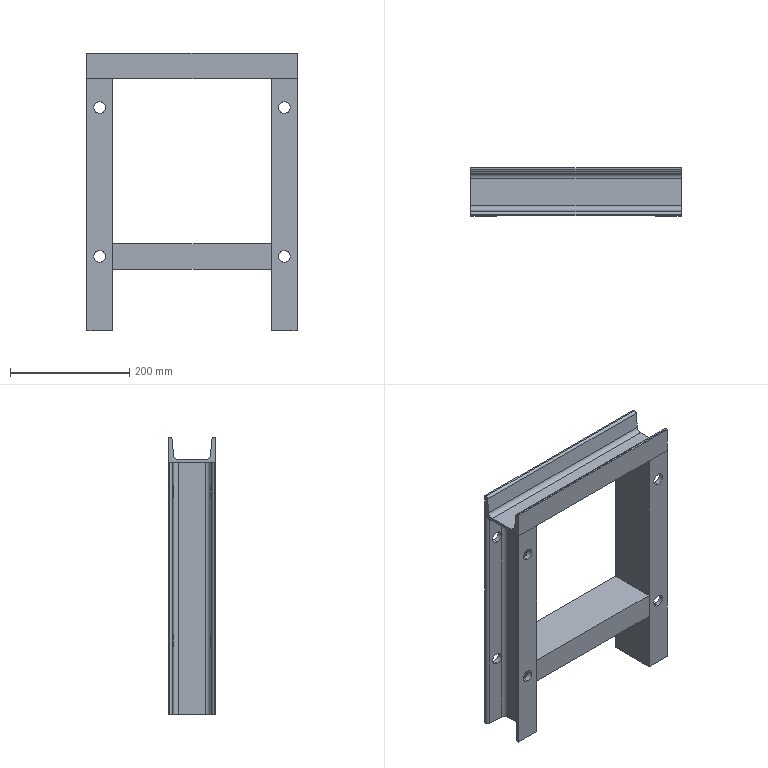Part | STEP file | Produce dryer motor mount_Default<As Machined> | 4 solids | 72 faces | box 353 x 80 x 466.5 mm | volume 1481860 mm3 | plane 40 | cylinder 32 | commonest cylinder face diameters 20 x16 8 x8 16 x8